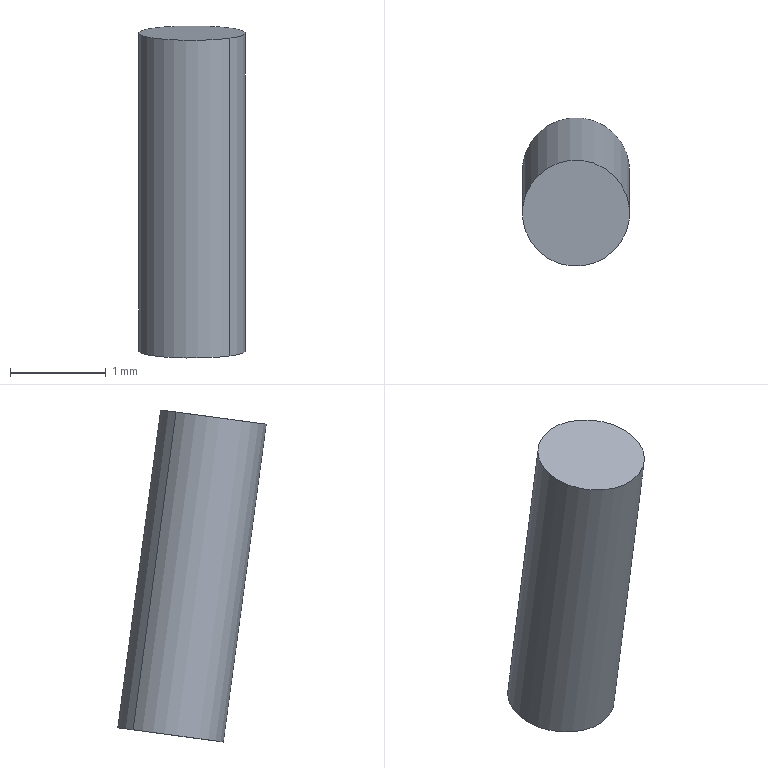Part | SolidWorks | features SplitBody 1 | 1 solid | 4 faces | box 1.118 x 1.555 x 3.463 mm | volume 3.28 mm3 | cylinder 2 | plane 2 | commonest cylinder face diameters 1.118 x2
STEP:
#1=CARTESIAN_POINT('',(578.968,442.515,-319.533));
#2=VERTEX_POINT('',#1);
#3=CARTESIAN_POINT('',(579.76,441.734,-319.638));
#4=VERTEX_POINT('',#3);
#5=CARTESIAN_POINT('',(579.364,442.124,-319.586));
#6=DIRECTION('',(0.,0.1337,-0.991));
#7=DIRECTION('',(-0.7089,0.6989,0.09427));
#8=AXIS2_PLACEMENT_3D('',#5,#6,#7);
#9=CIRCLE('',#8,0.5588);
#10=EDGE_CURVE('',#2,#4,#9,.T.);
#11=ORIENTED_EDGE('',*,*,#10,.F.);
#12=CARTESIAN_POINT('',(578.968,442.068,-316.219));
#13=VERTEX_POINT('',#12);
#14=CARTESIAN_POINT('',(578.968,442.515,-319.533));
#15=DIRECTION('',(0.,-0.1337,0.991));
#16=VECTOR('',#15,1000.);
#17=LINE('',#14,#16);
#18=EDGE_CURVE('',#2,#13,#17,.T.);
#19=ORIENTED_EDGE('',*,*,#18,.T.);
#20=CARTESIAN_POINT('',(579.76,441.287,-316.324));
#21=VERTEX_POINT('',#20);
#22=CARTESIAN_POINT('',(579.364,441.677,-316.272));
#23=DIRECTION('',(0.,0.1337,-0.991));
#24=DIRECTION('',(-0.7089,0.6989,0.09427));
#25=AXIS2_PLACEMENT_3D('',#22,#23,#24);
#26=CIRCLE('',#25,0.5588);
#27=EDGE_CURVE('',#13,#21,#26,.T.);
#28=ORIENTED_EDGE('',*,*,#27,.T.);
#29=CARTESIAN_POINT('',(579.76,441.734,-319.638));
#30=DIRECTION('',(0.,-0.1337,0.991));
#31=VECTOR('',#30,1000.);
#32=LINE('',#29,#31);
#33=EDGE_CURVE('',#4,#21,#32,.T.);
#34=ORIENTED_EDGE('',*,*,#33,.F.);
#35=EDGE_LOOP('',(#11,#19,#28,#34));
#36=FACE_OUTER_BOUND('',#35,.T.);
#37=CARTESIAN_POINT('',(579.364,442.124,-319.586));
#38=DIRECTION('',(0.,-0.1337,0.991));
#39=DIRECTION('',(0.7089,-0.6989,-0.09427));
#40=AXIS2_PLACEMENT_3D('',#37,#38,#39);
#41=CYLINDRICAL_SURFACE('',#40,0.5588);
#42=ADVANCED_FACE('',(#36),#41,.T.);
#43=ORIENTED_EDGE('',*,*,#18,.F.);
#44=CARTESIAN_POINT('',(579.364,442.124,-319.586));
#45=DIRECTION('',(0.,0.1337,-0.991));
#46=DIRECTION('',(-0.7089,0.6989,0.09427));
#47=AXIS2_PLACEMENT_3D('',#44,#45,#46);
#48=CIRCLE('',#47,0.5588);
#49=EDGE_CURVE('',#4,#2,#48,.T.);
#50=ORIENTED_EDGE('',*,*,#49,.F.);
#51=ORIENTED_EDGE('',*,*,#33,.T.);
#52=CARTESIAN_POINT('',(579.364,441.677,-316.272));
#53=DIRECTION('',(0.,0.1337,-0.991));
#54=DIRECTION('',(-0.7089,0.6989,0.09427));
#55=AXIS2_PLACEMENT_3D('',#52,#53,#54);
#56=CIRCLE('',#55,0.5588);
#57=EDGE_CURVE('',#21,#13,#56,.T.);
#58=ORIENTED_EDGE('',*,*,#57,.T.);
#59=EDGE_LOOP('',(#43,#50,#51,#58));
#60=FACE_OUTER_BOUND('',#59,.T.);
#61=CARTESIAN_POINT('',(579.364,442.124,-319.586));
#62=DIRECTION('',(0.,-0.1337,0.991));
#63=DIRECTION('',(0.7089,-0.6989,-0.09427));
#64=AXIS2_PLACEMENT_3D('',#61,#62,#63);
#65=CYLINDRICAL_SURFACE('',#64,0.5588);
#66=ADVANCED_FACE('',(#60),#65,.T.);
#67=ORIENTED_EDGE('',*,*,#49,.T.);
#68=ORIENTED_EDGE('',*,*,#10,.T.);
#69=EDGE_LOOP('',(#67,#68));
#70=FACE_OUTER_BOUND('',#69,.T.);
#71=CARTESIAN_POINT('',(579.364,442.124,-319.586));
#72=DIRECTION('',(0.,0.1337,-0.991));
#73=DIRECTION('',(-0.7089,0.6989,0.09427));
#74=AXIS2_PLACEMENT_3D('',#71,#72,#73);
#75=PLANE('',#74);
#76=ADVANCED_FACE('',(#70),#75,.T.);
#77=ORIENTED_EDGE('',*,*,#57,.F.);
#78=ORIENTED_EDGE('',*,*,#27,.F.);
#79=EDGE_LOOP('',(#77,#78));
#80=FACE_OUTER_BOUND('',#79,.T.);
#81=CARTESIAN_POINT('',(579.364,441.677,-316.272));
#82=DIRECTION('',(0.,0.1337,-0.991));
#83=DIRECTION('',(-0.7089,0.6989,0.09427));
#84=AXIS2_PLACEMENT_3D('',#81,#82,#83);
#85=PLANE('',#84);
#86=ADVANCED_FACE('',(#80),#85,.F.);
#87=CLOSED_SHELL('',(#42,#66,#76,#86));
#88=MANIFOLD_SOLID_BREP('',#87);
#89=CARTESIAN_POINT('',(0.,0.,0.));
#90=DIRECTION('',(0.,0.,1.));
#91=DIRECTION('',(1.,0.,0.));
#92=AXIS2_PLACEMENT_3D('',#89,#90,#91);
#93=(LENGTH_UNIT()NAMED_UNIT(*)SI_UNIT(.MILLI.,.METRE.));
#94=UNCERTAINTY_MEASURE_WITH_UNIT(LENGTH_MEASURE(0.00001),#93,'','');
#95=(NAMED_UNIT(*)PLANE_ANGLE_UNIT()SI_UNIT($,.RADIAN.));
#96=(NAMED_UNIT(*)SI_UNIT($,.STERADIAN.)SOLID_ANGLE_UNIT());
#97=(GEOMETRIC_REPRESENTATION_CONTEXT(3)GLOBAL_UNCERTAINTY_ASSIGNED_CONTEXT((#94))GLOBAL_UNIT_ASSIGNED_CONTEXT((#93,#95,#96))REPRESENTATION_CONTEXT('',''));
#98=ADVANCED_BREP_SHAPE_REPRESENTATION('',(#88,#92),#97);